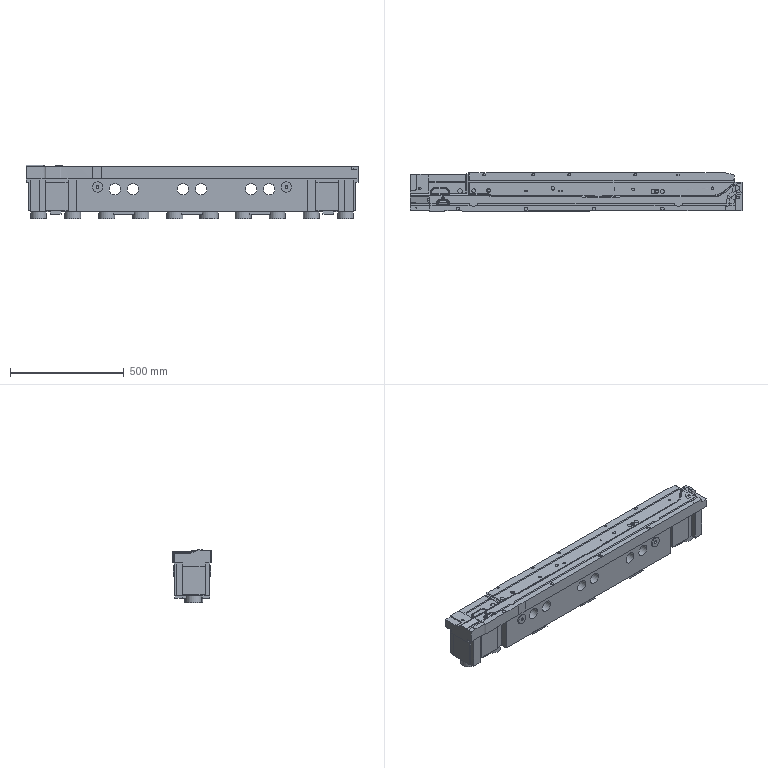Part | NX | features solid 2 | 1 solid | 334 faces | box 1460 x 169.867 x 235.617 mm | volume 41741038 mm3 | plane 143 | spline 121 | cylinder 62 | cone 6 | torus 1 | sphere 1 | commonest cylinder face diameters 12 x28 70 x9 50 x6 10 x4 40 x4 45 x4